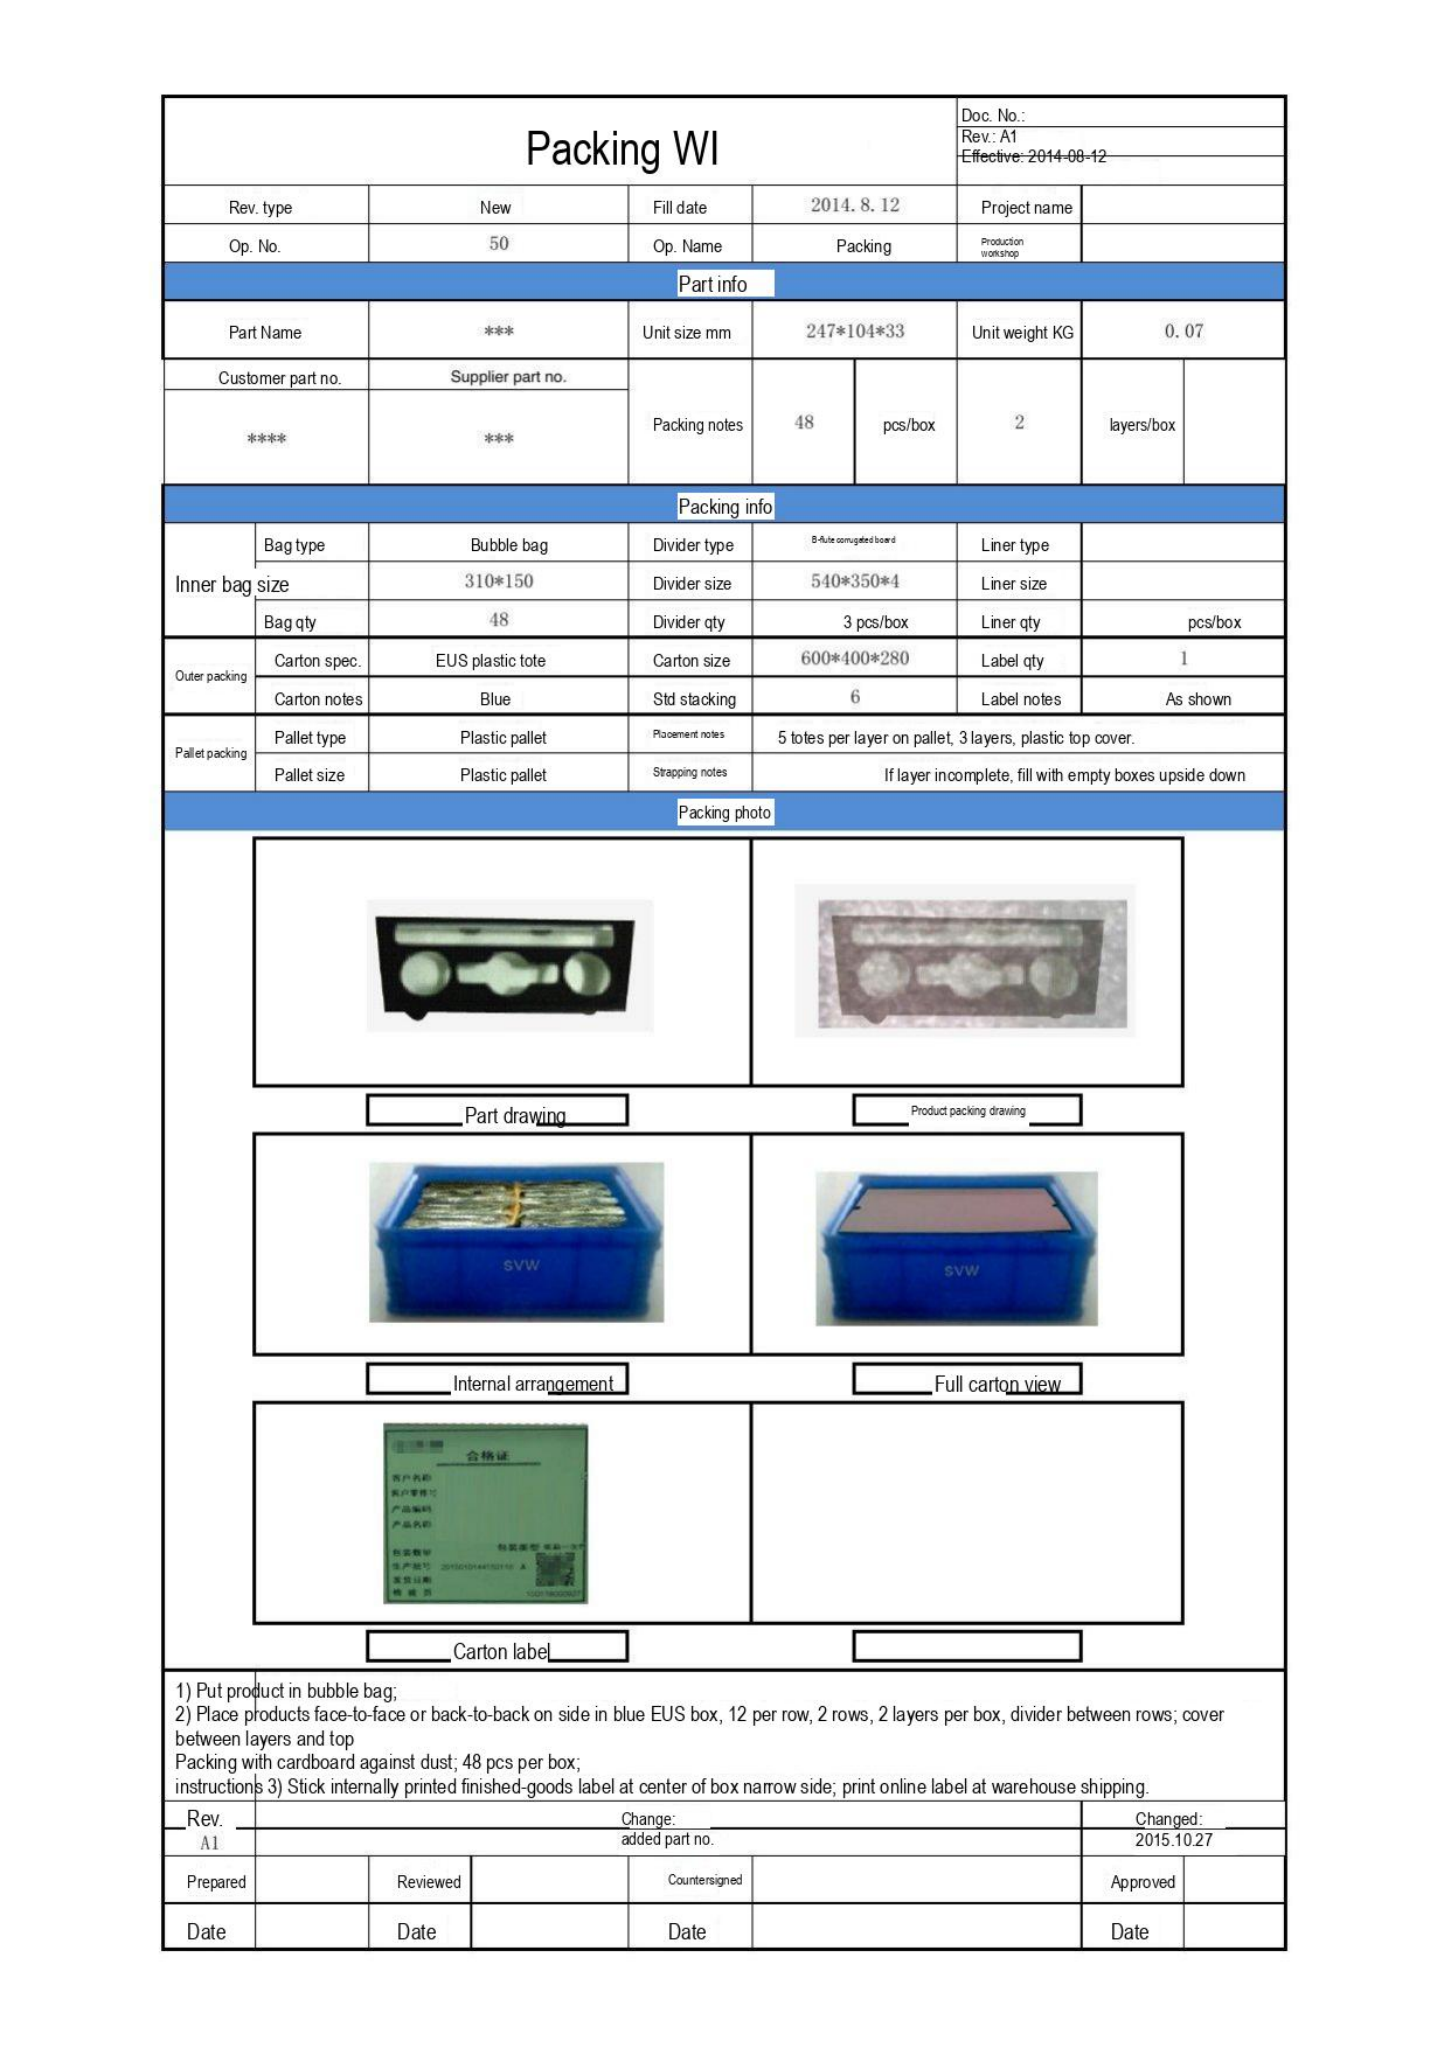# Packing WI

| Doc. No.: |
|---|
| Rev.: A1 |
| Effective: 2014-08-12 |

| Rev. type | New | Fill date | 2014. 8. 12 | Project name | |
|---|---|---|---|---|---|
| Op. No. | 50 | Op. Name | Packing | Production workshop | |

**Part info**

| Part Name | \*\*\* | Unit size mm | 247\*104\*33 | Unit weight KG | 0. 07 | |
|---|---|---|---|---|---|---|
| Customer part no. | Supplier part no. | Packing notes | 48 | pcs/box | 2 | layers/box |
| \*\*\*\* | \*\*\* | | | | | |

**Packing info**

| | | | | | | |
|---|---|---|---|---|---|---|
| Inner bag size | Bag type | Bubble bag | Divider type | B-flute corrugated board | Liner type | |
| | | 310\*150 | Divider size | 540\*350\*4 | Liner size | |
| | Bag qty | 48 | Divider qty | 3 pcs/box | Liner qty | pcs/box |
| Outer packing | Carton spec. | EUS plastic tote | Carton size | 600\*400\*280 | Label qty | 1 |
| | Carton notes | Blue | Std stacking | 6 | Label notes | As shown |
| Pallet packing | Pallet type | Plastic pallet | Placement notes | 5 totes per layer on pallet, 3 layers, plastic top cover. | | |
| | Pallet size | Plastic pallet | Strapping notes | If layer incomplete, fill with empty boxes upside down | | |

**Packing photo**

Part drawing

Product packing drawing

SVW

Internal arrangement

SVW

Full carton view

合格证

Carton label

1) Put product in bubble bag;
2) Place products face-to-face or back-to-back on side in blue EUS box, 12 per row, 2 rows, 2 layers per box, divider between rows; cover between layers and top
Packing with cardboard against dust; 48 pcs per box;
instructions 3) Stick internally printed finished-goods label at center of box narrow side; print online label at warehouse shipping.

| Rev. | Change: | Changed: |
|---|---|---|
| A1 | added part no. | 2015.10.27 |

| Prepared | | Reviewed | | Countersigned | | Approved | |
|---|---|---|---|---|---|---|---|
| Date | | Date | | Date | | Date | |